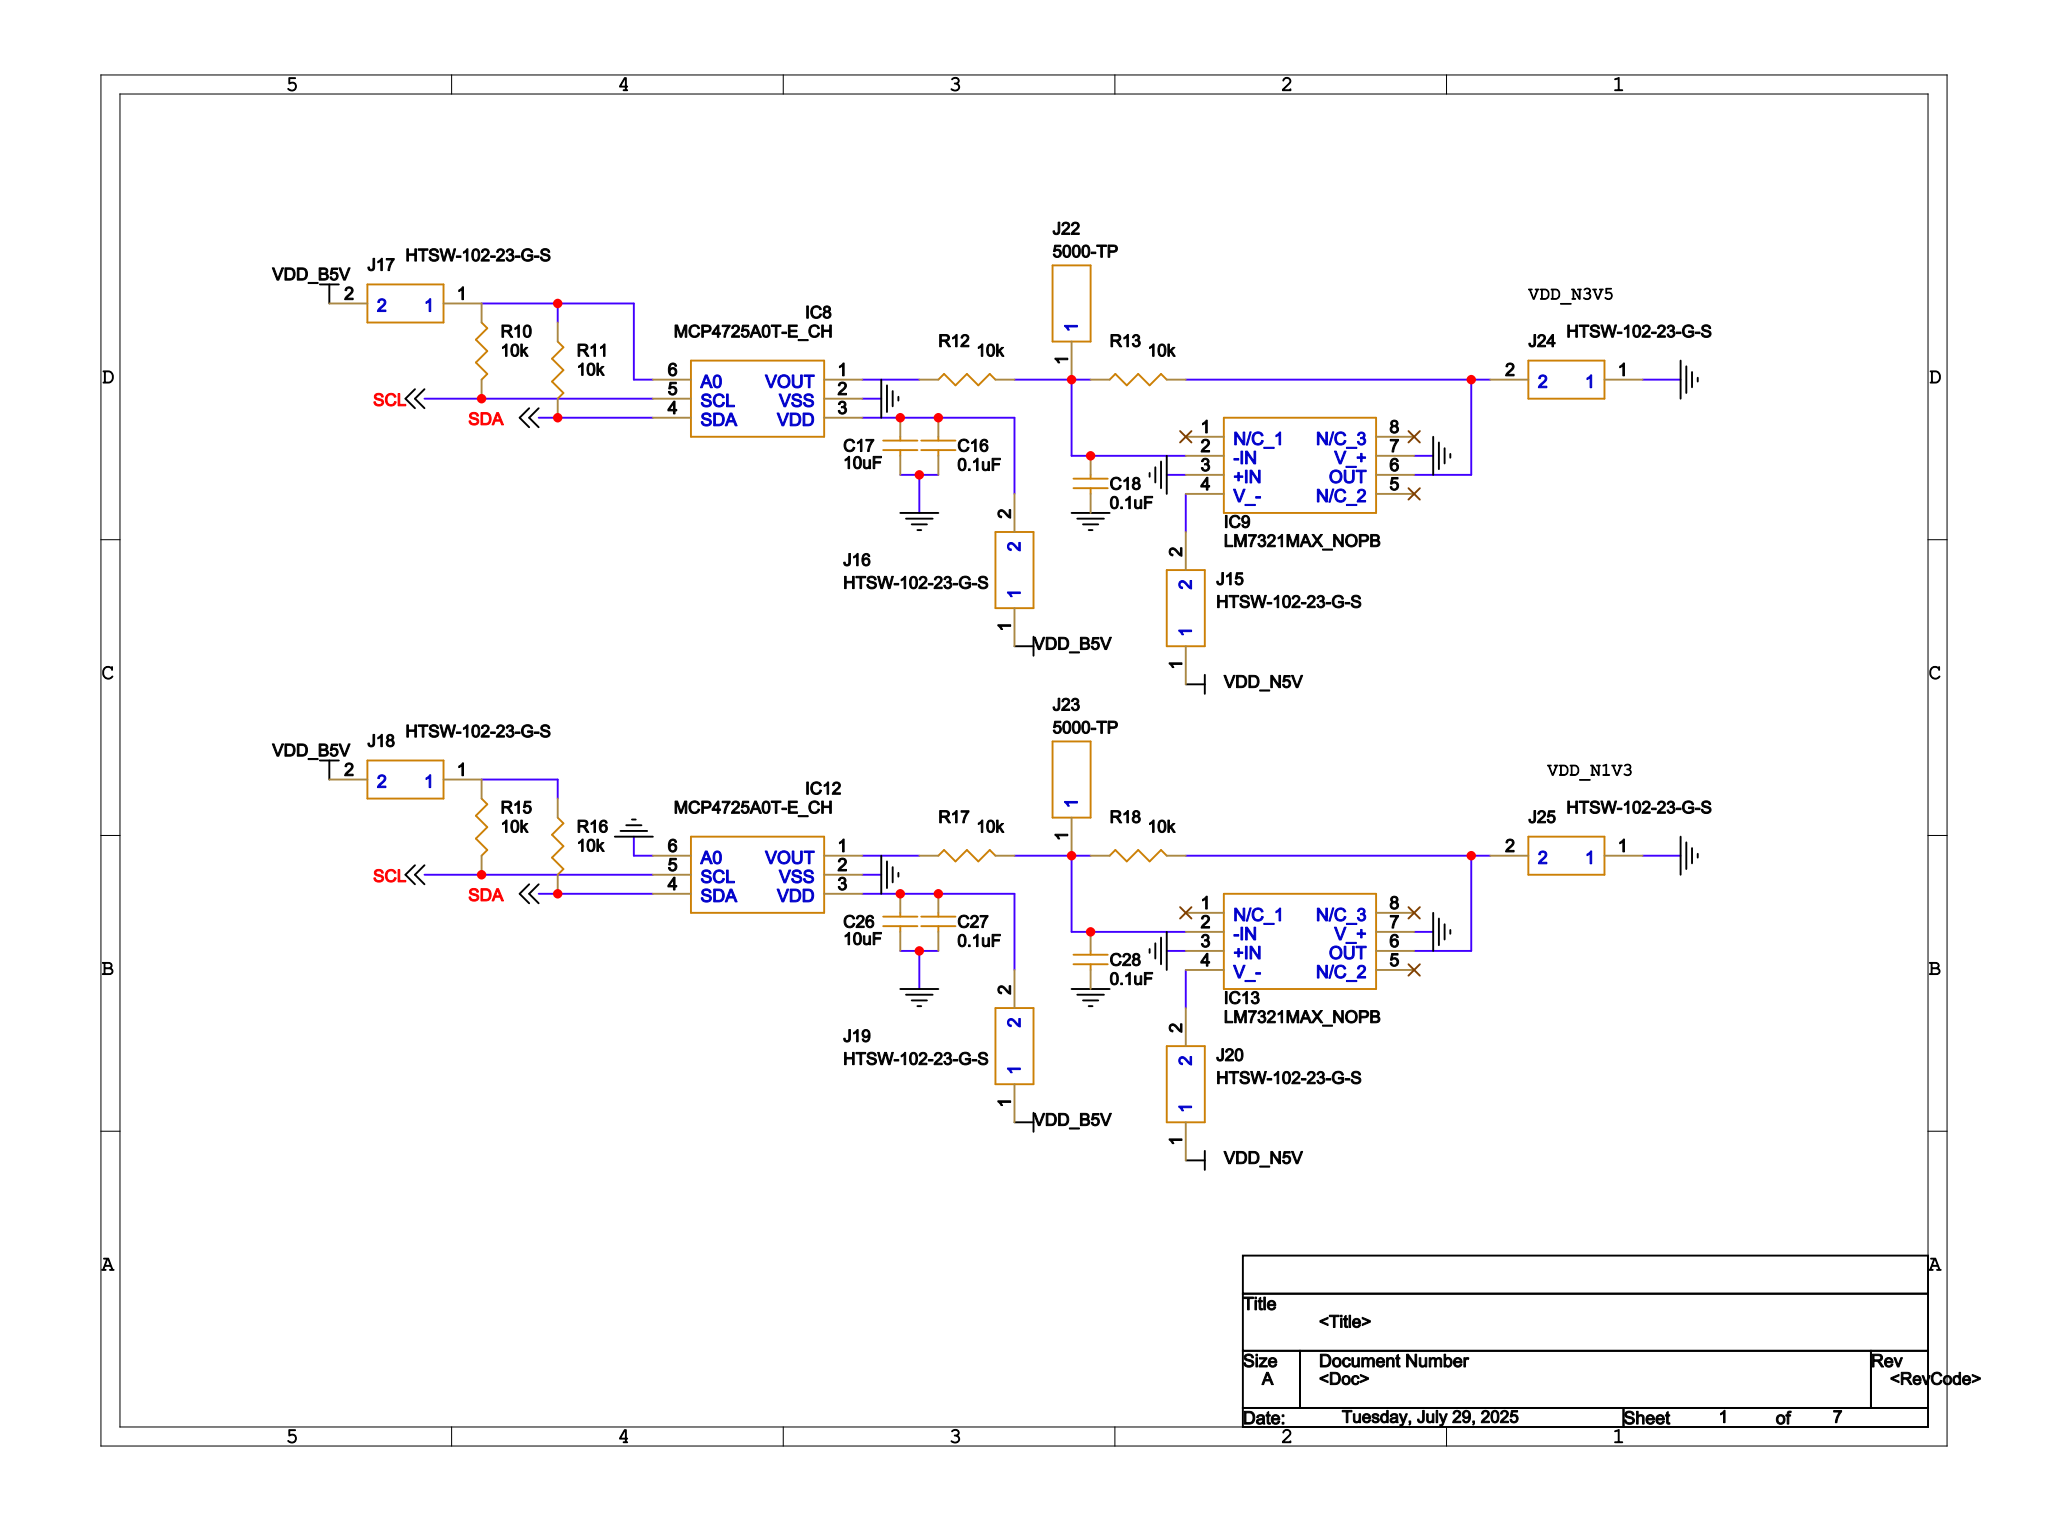Circuit board | Cadence Allegro | 93 parts | 49 nets | one sheet of the schematic
Parts on this sheet (reference | value | footprint):
C16 | 0.1uF | C0402
C17 | 10uF | C1210
C18 | 0.1uF | C0402
C26 | 10uF | C1210
C27 | 0.1uF | C0402
C28 | 0.1uF | C0402
IC8 | MCP4725A0T-E_CH | SOT95P270X145-6N
IC9 | LM7321MAX_NOPB | SOIC127P600X175-8N
IC12 | MCP4725A0T-E_CH | SOT95P270X145-6N
IC13 | LM7321MAX_NOPB | SOIC127P600X175-8N
J15 | HTSW-102-23-G-S | HDRV2W64P0X254_1X2_508X248X838P
J16 | HTSW-102-23-G-S | HDRV2W64P0X254_1X2_508X248X838P
J17 | HTSW-102-23-G-S | HDRV2W64P0X254_1X2_508X248X838P
J18 | HTSW-102-23-G-S | HDRV2W64P0X254_1X2_508X248X838P
J19 | HTSW-102-23-G-S | HDRV2W64P0X254_1X2_508X248X838P
J20 | HTSW-102-23-G-S | HDRV2W64P0X254_1X2_508X248X838P
J22 | 5000-TP | 5000
J23 | 5000-TP | 5000
J24 | HTSW-102-23-G-S | HDRV2W64P0X254_1X2_508X248X838P
J25 | HTSW-102-23-G-S | HDRV2W64P0X254_1X2_508X248X838P
R10 | 10k | R0402
R11 | 10k | R0402
R12 | 10k | R0402
R13 | 10k | R0402
R15 | 10k | R0402
R16 | 10k | R0402
R17 | 10k | R0402
R18 | 10k | R0402
Nets of these parts (net: part-pin ...):
GND: C16-2 C17-2 C18-2 C26-2 C27-2 C28-2 IC8-2 IC9-3 IC9-7 IC12-2 IC12-6 IC13-3 IC13-7 J24-1 J25-1
VDD_B5V: J16-1 J17-2 J18-2 J19-1
N06995: C16-1 C17-1 IC8-3 J16-2
VDD_N5V: J15-1 J20-1
N11311: C26-1 C27-1 IC12-3 J19-2
SCL: IC8-5 IC12-5 R10-2 R15-2
SDA: IC8-4 IC12-4 R11-2 R16-2
N07127: C18-1 IC9-2 J22-1 R12-2 R13-1
N11263: C28-1 IC13-2 J23-1 R17-2 R18-1
N06846: IC8-6 J17-1 R10-1 R11-1
N06991: IC8-1 R12-1
N07296: IC9-6 J24-2 R13-2
N11131: J18-1 R15-1 R16-1
N11255: IC12-1 R17-1
N11271: IC13-6 J25-2 R18-2
N11439: IC13-4 J20-2
N07252: IC9-4 J15-2